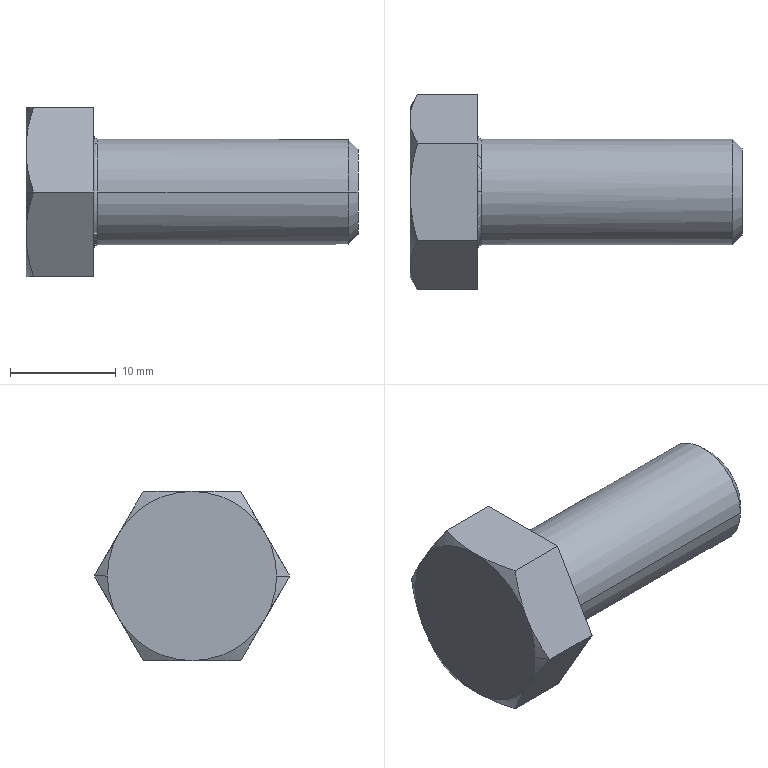Part | STEP file | KS B 1002 - C  M 10 x 25 | 1 solid | 23 faces | box 31.4 x 18.475 x 16 mm | volume 3367 mm3 | cone 10 | plane 9 | torus 2 | cylinder 2 | commonest cylinder face diameters 10 x2